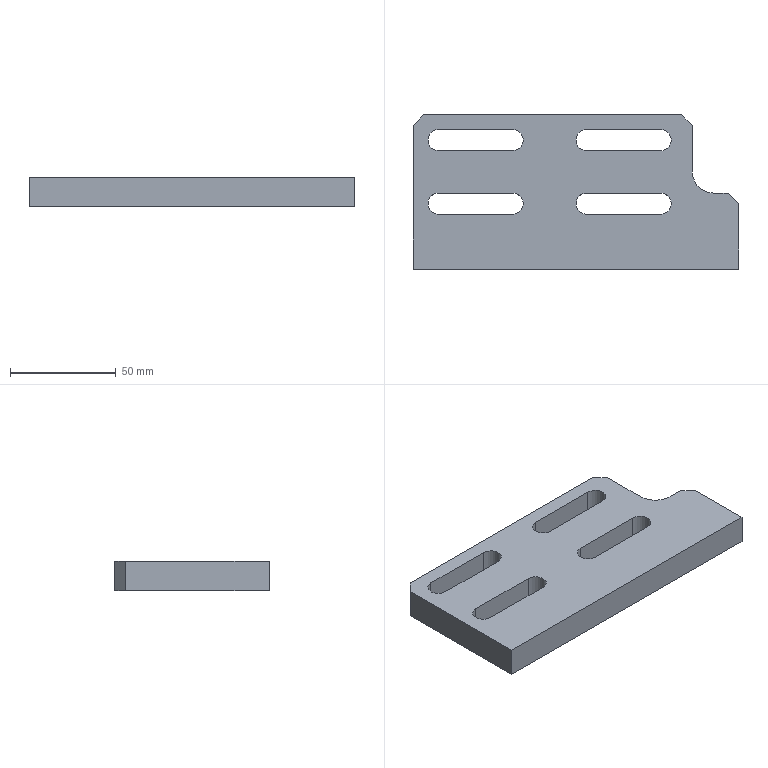Part | STEP file | [02] | 1 solid | 28 faces | box 154 x 73 x 14 mm | volume 121769 mm3 | plane 19 | cylinder 9 | commonest cylinder face diameters 10 x8 20 x1
STEP:
#1=CARTESIAN_POINT('',(15.,66.,14.));
#2=VERTEX_POINT('',#1);
#3=CARTESIAN_POINT('',(50.,66.,14.));
#4=VERTEX_POINT('',#3);
#5=CARTESIAN_POINT('',(32.5,66.,14.));
#6=DIRECTION('',(1.,0.,0.));
#7=VECTOR('',#6,1000.);
#8=LINE('',#5,#7);
#9=EDGE_CURVE('',#2,#4,#8,.T.);
#10=ORIENTED_EDGE('',*,*,#9,.T.);
#11=CARTESIAN_POINT('',(50.,56.,14.));
#12=VERTEX_POINT('',#11);
#13=CARTESIAN_POINT('',(50.,61.,14.));
#14=DIRECTION('',(0.,0.,-1.));
#15=DIRECTION('',(0.,1.,0.));
#16=AXIS2_PLACEMENT_3D('',#13,#14,#15);
#17=CIRCLE('',#16,5.);
#18=EDGE_CURVE('',#4,#12,#17,.T.);
#19=ORIENTED_EDGE('',*,*,#18,.T.);
#20=CARTESIAN_POINT('',(15.,56.,14.));
#21=VERTEX_POINT('',#20);
#22=CARTESIAN_POINT('',(32.5,56.,14.));
#23=DIRECTION('',(-1.,0.,0.));
#24=VECTOR('',#23,1000.);
#25=LINE('',#22,#24);
#26=EDGE_CURVE('',#12,#21,#25,.T.);
#27=ORIENTED_EDGE('',*,*,#26,.T.);
#28=CARTESIAN_POINT('',(15.,61.,14.));
#29=DIRECTION('',(0.,0.,-1.));
#30=DIRECTION('',(0.,1.,0.));
#31=AXIS2_PLACEMENT_3D('',#28,#29,#30);
#32=CIRCLE('',#31,5.);
#33=EDGE_CURVE('',#21,#2,#32,.T.);
#34=ORIENTED_EDGE('',*,*,#33,.T.);
#35=EDGE_LOOP('',(#10,#19,#27,#34));
#36=FACE_BOUND('',#35,.T.);
#37=CARTESIAN_POINT('',(15.,36.,14.));
#38=VERTEX_POINT('',#37);
#39=CARTESIAN_POINT('',(50.,36.,14.));
#40=VERTEX_POINT('',#39);
#41=CARTESIAN_POINT('',(32.5,36.,14.));
#42=DIRECTION('',(1.,0.,0.));
#43=VECTOR('',#42,1000.);
#44=LINE('',#41,#43);
#45=EDGE_CURVE('',#38,#40,#44,.T.);
#46=ORIENTED_EDGE('',*,*,#45,.T.);
#47=CARTESIAN_POINT('',(50.,26.,14.));
#48=VERTEX_POINT('',#47);
#49=CARTESIAN_POINT('',(50.,31.,14.));
#50=DIRECTION('',(0.,0.,-1.));
#51=DIRECTION('',(0.,1.,0.));
#52=AXIS2_PLACEMENT_3D('',#49,#50,#51);
#53=CIRCLE('',#52,5.);
#54=EDGE_CURVE('',#40,#48,#53,.T.);
#55=ORIENTED_EDGE('',*,*,#54,.T.);
#56=CARTESIAN_POINT('',(15.,26.,14.));
#57=VERTEX_POINT('',#56);
#58=CARTESIAN_POINT('',(32.5,26.,14.));
#59=DIRECTION('',(-1.,0.,0.));
#60=VECTOR('',#59,1000.);
#61=LINE('',#58,#60);
#62=EDGE_CURVE('',#48,#57,#61,.T.);
#63=ORIENTED_EDGE('',*,*,#62,.T.);
#64=CARTESIAN_POINT('',(15.,31.,14.));
#65=DIRECTION('',(0.,0.,-1.));
#66=DIRECTION('',(0.,1.,0.));
#67=AXIS2_PLACEMENT_3D('',#64,#65,#66);
#68=CIRCLE('',#67,5.);
#69=EDGE_CURVE('',#57,#38,#68,.T.);
#70=ORIENTED_EDGE('',*,*,#69,.T.);
#71=EDGE_LOOP('',(#46,#55,#63,#70));
#72=FACE_BOUND('',#71,.T.);
#73=CARTESIAN_POINT('',(85.,66.,14.));
#74=VERTEX_POINT('',#73);
#75=CARTESIAN_POINT('',(120.,66.,14.));
#76=VERTEX_POINT('',#75);
#77=CARTESIAN_POINT('',(102.5,66.,14.));
#78=DIRECTION('',(1.,0.,0.));
#79=VECTOR('',#78,1000.);
#80=LINE('',#77,#79);
#81=EDGE_CURVE('',#74,#76,#80,.T.);
#82=ORIENTED_EDGE('',*,*,#81,.T.);
#83=CARTESIAN_POINT('',(120.,56.,14.));
#84=VERTEX_POINT('',#83);
#85=CARTESIAN_POINT('',(120.,61.,14.));
#86=DIRECTION('',(0.,0.,-1.));
#87=DIRECTION('',(0.,1.,0.));
#88=AXIS2_PLACEMENT_3D('',#85,#86,#87);
#89=CIRCLE('',#88,5.);
#90=EDGE_CURVE('',#76,#84,#89,.T.);
#91=ORIENTED_EDGE('',*,*,#90,.T.);
#92=CARTESIAN_POINT('',(85.,56.,14.));
#93=VERTEX_POINT('',#92);
#94=CARTESIAN_POINT('',(102.5,56.,14.));
#95=DIRECTION('',(-1.,0.,0.));
#96=VECTOR('',#95,1000.);
#97=LINE('',#94,#96);
#98=EDGE_CURVE('',#84,#93,#97,.T.);
#99=ORIENTED_EDGE('',*,*,#98,.T.);
#100=CARTESIAN_POINT('',(85.,61.,14.));
#101=DIRECTION('',(0.,0.,-1.));
#102=DIRECTION('',(0.,1.,0.));
#103=AXIS2_PLACEMENT_3D('',#100,#101,#102);
#104=CIRCLE('',#103,5.);
#105=EDGE_CURVE('',#93,#74,#104,.T.);
#106=ORIENTED_EDGE('',*,*,#105,.T.);
#107=EDGE_LOOP('',(#82,#91,#99,#106));
#108=FACE_BOUND('',#107,.T.);
#109=CARTESIAN_POINT('',(85.,36.,14.));
#110=VERTEX_POINT('',#109);
#111=CARTESIAN_POINT('',(120.,36.,14.));
#112=VERTEX_POINT('',#111);
#113=CARTESIAN_POINT('',(102.5,36.,14.));
#114=DIRECTION('',(1.,0.,0.));
#115=VECTOR('',#114,1000.);
#116=LINE('',#113,#115);
#117=EDGE_CURVE('',#110,#112,#116,.T.);
#118=ORIENTED_EDGE('',*,*,#117,.T.);
#119=CARTESIAN_POINT('',(120.,26.,14.));
#120=VERTEX_POINT('',#119);
#121=CARTESIAN_POINT('',(120.,31.,14.));
#122=DIRECTION('',(0.,0.,-1.));
#123=DIRECTION('',(0.,1.,0.));
#124=AXIS2_PLACEMENT_3D('',#121,#122,#123);
#125=CIRCLE('',#124,5.);
#126=EDGE_CURVE('',#112,#120,#125,.T.);
#127=ORIENTED_EDGE('',*,*,#126,.T.);
#128=CARTESIAN_POINT('',(85.,26.,14.));
#129=VERTEX_POINT('',#128);
#130=CARTESIAN_POINT('',(102.5,26.,14.));
#131=DIRECTION('',(-1.,0.,0.));
#132=VECTOR('',#131,1000.);
#133=LINE('',#130,#132);
#134=EDGE_CURVE('',#120,#129,#133,.T.);
#135=ORIENTED_EDGE('',*,*,#134,.T.);
#136=CARTESIAN_POINT('',(85.,31.,14.));
#137=DIRECTION('',(0.,0.,-1.));
#138=DIRECTION('',(0.,1.,0.));
#139=AXIS2_PLACEMENT_3D('',#136,#137,#138);
#140=CIRCLE('',#139,5.);
#141=EDGE_CURVE('',#129,#110,#140,.T.);
#142=ORIENTED_EDGE('',*,*,#141,.T.);
#143=EDGE_LOOP('',(#118,#127,#135,#142));
#144=FACE_BOUND('',#143,.T.);
#145=CARTESIAN_POINT('',(135.,46.,14.));
#146=VERTEX_POINT('',#145);
#147=CARTESIAN_POINT('',(135.,68.,14.));
#148=VERTEX_POINT('',#147);
#149=CARTESIAN_POINT('',(135.,54.5,14.));
#150=DIRECTION('',(0.,1.,0.));
#151=VECTOR('',#150,1000.);
#152=LINE('',#149,#151);
#153=EDGE_CURVE('',#146,#148,#152,.T.);
#154=ORIENTED_EDGE('',*,*,#153,.T.);
#155=CARTESIAN_POINT('',(130.,73.,14.));
#156=VERTEX_POINT('',#155);
#157=CARTESIAN_POINT('',(123.25,79.75,14.));
#158=DIRECTION('',(-0.7071,0.7071,0.));
#159=VECTOR('',#158,1000.);
#160=LINE('',#157,#159);
#161=EDGE_CURVE('',#148,#156,#160,.T.);
#162=ORIENTED_EDGE('',*,*,#161,.T.);
#163=CARTESIAN_POINT('',(8.,73.,14.));
#164=VERTEX_POINT('',#163);
#165=CARTESIAN_POINT('',(80.,73.,14.));
#166=DIRECTION('',(1.,0.,0.));
#167=VECTOR('',#166,1000.);
#168=LINE('',#165,#167);
#169=EDGE_CURVE('',#164,#156,#168,.T.);
#170=ORIENTED_EDGE('',*,*,#169,.F.);
#171=CARTESIAN_POINT('',(3.,68.,14.));
#172=VERTEX_POINT('',#171);
#173=CARTESIAN_POINT('',(25.75,90.75,14.));
#174=DIRECTION('',(-0.7071,-0.7071,0.));
#175=VECTOR('',#174,1000.);
#176=LINE('',#173,#175);
#177=EDGE_CURVE('',#164,#172,#176,.T.);
#178=ORIENTED_EDGE('',*,*,#177,.T.);
#179=CARTESIAN_POINT('',(3.,0.,14.));
#180=VERTEX_POINT('',#179);
#181=CARTESIAN_POINT('',(3.,36.5,14.));
#182=DIRECTION('',(0.,1.,0.));
#183=VECTOR('',#182,1000.);
#184=LINE('',#181,#183);
#185=EDGE_CURVE('',#180,#172,#184,.T.);
#186=ORIENTED_EDGE('',*,*,#185,.F.);
#187=CARTESIAN_POINT('',(157.,0.,14.));
#188=VERTEX_POINT('',#187);
#189=CARTESIAN_POINT('',(80.,0.,14.));
#190=DIRECTION('',(-1.,0.,0.));
#191=VECTOR('',#190,1000.);
#192=LINE('',#189,#191);
#193=EDGE_CURVE('',#188,#180,#192,.T.);
#194=ORIENTED_EDGE('',*,*,#193,.F.);
#195=CARTESIAN_POINT('',(157.,31.,14.));
#196=VERTEX_POINT('',#195);
#197=CARTESIAN_POINT('',(157.,36.5,14.));
#198=DIRECTION('',(0.,-1.,0.));
#199=VECTOR('',#198,1000.);
#200=LINE('',#197,#199);
#201=EDGE_CURVE('',#196,#188,#200,.T.);
#202=ORIENTED_EDGE('',*,*,#201,.F.);
#203=CARTESIAN_POINT('',(152.,36.,14.));
#204=VERTEX_POINT('',#203);
#205=CARTESIAN_POINT('',(115.75,72.25,14.));
#206=DIRECTION('',(-0.7071,0.7071,0.));
#207=VECTOR('',#206,1000.);
#208=LINE('',#205,#207);
#209=EDGE_CURVE('',#196,#204,#208,.T.);
#210=ORIENTED_EDGE('',*,*,#209,.T.);
#211=CARTESIAN_POINT('',(145.,36.,14.));
#212=VERTEX_POINT('',#211);
#213=CARTESIAN_POINT('',(146.,36.,14.));
#214=DIRECTION('',(-1.,0.,0.));
#215=VECTOR('',#214,1000.);
#216=LINE('',#213,#215);
#217=EDGE_CURVE('',#204,#212,#216,.T.);
#218=ORIENTED_EDGE('',*,*,#217,.T.);
#219=CARTESIAN_POINT('',(145.,46.,14.));
#220=DIRECTION('',(0.,0.,-1.));
#221=DIRECTION('',(0.,-1.,0.));
#222=AXIS2_PLACEMENT_3D('',#219,#220,#221);
#223=CIRCLE('',#222,10.);
#224=EDGE_CURVE('',#212,#146,#223,.T.);
#225=ORIENTED_EDGE('',*,*,#224,.T.);
#226=EDGE_LOOP('',(#154,#162,#170,#178,#186,#194,#202,#210,#218,#225));
#227=FACE_OUTER_BOUND('',#226,.T.);
#228=CARTESIAN_POINT('',(80.,36.5,14.));
#229=DIRECTION('',(0.,0.,1.));
#230=DIRECTION('',(0.,-1.,0.));
#231=AXIS2_PLACEMENT_3D('',#228,#229,#230);
#232=PLANE('',#231);
#233=ADVANCED_FACE('',(#36,#72,#108,#144,#227),#232,.T.);
#234=CARTESIAN_POINT('',(15.,56.,0.));
#235=VERTEX_POINT('',#234);
#236=CARTESIAN_POINT('',(50.,56.,0.));
#237=VERTEX_POINT('',#236);
#238=CARTESIAN_POINT('',(32.5,56.,0.));
#239=DIRECTION('',(1.,0.,0.));
#240=VECTOR('',#239,1000.);
#241=LINE('',#238,#240);
#242=EDGE_CURVE('',#235,#237,#241,.T.);
#243=ORIENTED_EDGE('',*,*,#242,.T.);
#244=CARTESIAN_POINT('',(50.,66.,0.));
#245=VERTEX_POINT('',#244);
#246=CARTESIAN_POINT('',(50.,61.,0.));
#247=DIRECTION('',(0.,0.,1.));
#248=DIRECTION('',(0.,-1.,0.));
#249=AXIS2_PLACEMENT_3D('',#246,#247,#248);
#250=CIRCLE('',#249,5.);
#251=EDGE_CURVE('',#237,#245,#250,.T.);
#252=ORIENTED_EDGE('',*,*,#251,.T.);
#253=CARTESIAN_POINT('',(15.,66.,0.));
#254=VERTEX_POINT('',#253);
#255=CARTESIAN_POINT('',(32.5,66.,0.));
#256=DIRECTION('',(-1.,0.,0.));
#257=VECTOR('',#256,1000.);
#258=LINE('',#255,#257);
#259=EDGE_CURVE('',#245,#254,#258,.T.);
#260=ORIENTED_EDGE('',*,*,#259,.T.);
#261=CARTESIAN_POINT('',(15.,61.,0.));
#262=DIRECTION('',(0.,0.,1.));
#263=DIRECTION('',(0.,-1.,0.));
#264=AXIS2_PLACEMENT_3D('',#261,#262,#263);
#265=CIRCLE('',#264,5.);
#266=EDGE_CURVE('',#254,#235,#265,.T.);
#267=ORIENTED_EDGE('',*,*,#266,.T.);
#268=EDGE_LOOP('',(#243,#252,#260,#267));
#269=FACE_BOUND('',#268,.T.);
#270=CARTESIAN_POINT('',(15.,26.,0.));
#271=VERTEX_POINT('',#270);
#272=CARTESIAN_POINT('',(50.,26.,0.));
#273=VERTEX_POINT('',#272);
#274=CARTESIAN_POINT('',(32.5,26.,0.));
#275=DIRECTION('',(1.,0.,0.));
#276=VECTOR('',#275,1000.);
#277=LINE('',#274,#276);
#278=EDGE_CURVE('',#271,#273,#277,.T.);
#279=ORIENTED_EDGE('',*,*,#278,.T.);
#280=CARTESIAN_POINT('',(50.,36.,0.));
#281=VERTEX_POINT('',#280);
#282=CARTESIAN_POINT('',(50.,31.,0.));
#283=DIRECTION('',(0.,0.,1.));
#284=DIRECTION('',(0.,-1.,0.));
#285=AXIS2_PLACEMENT_3D('',#282,#283,#284);
#286=CIRCLE('',#285,5.);
#287=EDGE_CURVE('',#273,#281,#286,.T.);
#288=ORIENTED_EDGE('',*,*,#287,.T.);
#289=CARTESIAN_POINT('',(15.,36.,0.));
#290=VERTEX_POINT('',#289);
#291=CARTESIAN_POINT('',(32.5,36.,0.));
#292=DIRECTION('',(-1.,0.,0.));
#293=VECTOR('',#292,1000.);
#294=LINE('',#291,#293);
#295=EDGE_CURVE('',#281,#290,#294,.T.);
#296=ORIENTED_EDGE('',*,*,#295,.T.);
#297=CARTESIAN_POINT('',(15.,31.,0.));
#298=DIRECTION('',(0.,0.,1.));
#299=DIRECTION('',(0.,-1.,0.));
#300=AXIS2_PLACEMENT_3D('',#297,#298,#299);
#301=CIRCLE('',#300,5.);
#302=EDGE_CURVE('',#290,#271,#301,.T.);
#303=ORIENTED_EDGE('',*,*,#302,.T.);
#304=EDGE_LOOP('',(#279,#288,#296,#303));
#305=FACE_BOUND('',#304,.T.);
#306=CARTESIAN_POINT('',(85.,56.,0.));
#307=VERTEX_POINT('',#306);
#308=CARTESIAN_POINT('',(120.,56.,0.));
#309=VERTEX_POINT('',#308);
#310=CARTESIAN_POINT('',(102.5,56.,0.));
#311=DIRECTION('',(1.,0.,0.));
#312=VECTOR('',#311,1000.);
#313=LINE('',#310,#312);
#314=EDGE_CURVE('',#307,#309,#313,.T.);
#315=ORIENTED_EDGE('',*,*,#314,.T.);
#316=CARTESIAN_POINT('',(120.,66.,0.));
#317=VERTEX_POINT('',#316);
#318=CARTESIAN_POINT('',(120.,61.,0.));
#319=DIRECTION('',(0.,0.,1.));
#320=DIRECTION('',(0.,-1.,0.));
#321=AXIS2_PLACEMENT_3D('',#318,#319,#320);
#322=CIRCLE('',#321,5.);
#323=EDGE_CURVE('',#309,#317,#322,.T.);
#324=ORIENTED_EDGE('',*,*,#323,.T.);
#325=CARTESIAN_POINT('',(85.,66.,0.));
#326=VERTEX_POINT('',#325);
#327=CARTESIAN_POINT('',(102.5,66.,0.));
#328=DIRECTION('',(-1.,0.,0.));
#329=VECTOR('',#328,1000.);
#330=LINE('',#327,#329);
#331=EDGE_CURVE('',#317,#326,#330,.T.);
#332=ORIENTED_EDGE('',*,*,#331,.T.);
#333=CARTESIAN_POINT('',(85.,61.,0.));
#334=DIRECTION('',(0.,0.,1.));
#335=DIRECTION('',(0.,-1.,0.));
#336=AXIS2_PLACEMENT_3D('',#333,#334,#335);
#337=CIRCLE('',#336,5.);
#338=EDGE_CURVE('',#326,#307,#337,.T.);
#339=ORIENTED_EDGE('',*,*,#338,.T.);
#340=EDGE_LOOP('',(#315,#324,#332,#339));
#341=FACE_BOUND('',#340,.T.);
#342=CARTESIAN_POINT('',(85.,26.,0.));
#343=VERTEX_POINT('',#342);
#344=CARTESIAN_POINT('',(120.,26.,0.));
#345=VERTEX_POINT('',#344);
#346=CARTESIAN_POINT('',(102.5,26.,0.));
#347=DIRECTION('',(1.,0.,0.));
#348=VECTOR('',#347,1000.);
#349=LINE('',#346,#348);
#350=EDGE_CURVE('',#343,#345,#349,.T.);
#351=ORIENTED_EDGE('',*,*,#350,.T.);
#352=CARTESIAN_POINT('',(120.,36.,0.));
#353=VERTEX_POINT('',#352);
#354=CARTESIAN_POINT('',(120.,31.,0.));
#355=DIRECTION('',(0.,0.,1.));
#356=DIRECTION('',(0.,-1.,0.));
#357=AXIS2_PLACEMENT_3D('',#354,#355,#356);
#358=CIRCLE('',#357,5.);
#359=EDGE_CURVE('',#345,#353,#358,.T.);
#360=ORIENTED_EDGE('',*,*,#359,.T.);
#361=CARTESIAN_POINT('',(85.,36.,0.));
#362=VERTEX_POINT('',#361);
#363=CARTESIAN_POINT('',(102.5,36.,0.));
#364=DIRECTION('',(-1.,0.,0.));
#365=VECTOR('',#364,1000.);
#366=LINE('',#363,#365);
#367=EDGE_CURVE('',#353,#362,#366,.T.);
#368=ORIENTED_EDGE('',*,*,#367,.T.);
#369=CARTESIAN_POINT('',(85.,31.,0.));
#370=DIRECTION('',(0.,0.,1.));
#371=DIRECTION('',(0.,-1.,0.));
#372=AXIS2_PLACEMENT_3D('',#369,#370,#371);
#373=CIRCLE('',#372,5.);
#374=EDGE_CURVE('',#362,#343,#373,.T.);
#375=ORIENTED_EDGE('',*,*,#374,.T.);
#376=EDGE_LOOP('',(#351,#360,#368,#375));
#377=FACE_BOUND('',#376,.T.);
#378=CARTESIAN_POINT('',(130.,73.,0.));
#379=VERTEX_POINT('',#378);
#380=CARTESIAN_POINT('',(8.,73.,0.));
#381=VERTEX_POINT('',#380);
#382=CARTESIAN_POINT('',(80.,73.,0.));
#383=DIRECTION('',(-1.,0.,0.));
#384=VECTOR('',#383,1000.);
#385=LINE('',#382,#384);
#386=EDGE_CURVE('',#379,#381,#385,.T.);
#387=ORIENTED_EDGE('',*,*,#386,.F.);
#388=CARTESIAN_POINT('',(135.,68.,0.));
#389=VERTEX_POINT('',#388);
#390=CARTESIAN_POINT('',(123.25,79.75,0.));
#391=DIRECTION('',(0.7071,-0.7071,0.));
#392=VECTOR('',#391,1000.);
#393=LINE('',#390,#392);
#394=EDGE_CURVE('',#379,#389,#393,.T.);
#395=ORIENTED_EDGE('',*,*,#394,.T.);
#396=CARTESIAN_POINT('',(135.,46.,0.));
#397=VERTEX_POINT('',#396);
#398=CARTESIAN_POINT('',(135.,54.5,0.));
#399=DIRECTION('',(0.,-1.,0.));
#400=VECTOR('',#399,1000.);
#401=LINE('',#398,#400);
#402=EDGE_CURVE('',#389,#397,#401,.T.);
#403=ORIENTED_EDGE('',*,*,#402,.T.);
#404=CARTESIAN_POINT('',(145.,36.,0.));
#405=VERTEX_POINT('',#404);
#406=CARTESIAN_POINT('',(145.,46.,0.));
#407=DIRECTION('',(0.,0.,1.));
#408=DIRECTION('',(0.,1.,0.));
#409=AXIS2_PLACEMENT_3D('',#406,#407,#408);
#410=CIRCLE('',#409,10.);
#411=EDGE_CURVE('',#397,#405,#410,.T.);
#412=ORIENTED_EDGE('',*,*,#411,.T.);
#413=CARTESIAN_POINT('',(152.,36.,0.));
#414=VERTEX_POINT('',#413);
#415=CARTESIAN_POINT('',(146.,36.,0.));
#416=DIRECTION('',(1.,0.,0.));
#417=VECTOR('',#416,1000.);
#418=LINE('',#415,#417);
#419=EDGE_CURVE('',#405,#414,#418,.T.);
#420=ORIENTED_EDGE('',*,*,#419,.T.);
#421=CARTESIAN_POINT('',(157.,31.,0.));
#422=VERTEX_POINT('',#421);
#423=CARTESIAN_POINT('',(115.75,72.25,0.));
#424=DIRECTION('',(0.7071,-0.7071,0.));
#425=VECTOR('',#424,1000.);
#426=LINE('',#423,#425);
#427=EDGE_CURVE('',#414,#422,#426,.T.);
#428=ORIENTED_EDGE('',*,*,#427,.T.);
#429=CARTESIAN_POINT('',(157.,0.,0.));
#430=VERTEX_POINT('',#429);
#431=CARTESIAN_POINT('',(157.,36.5,0.));
#432=DIRECTION('',(0.,1.,0.));
#433=VECTOR('',#432,1000.);
#434=LINE('',#431,#433);
#435=EDGE_CURVE('',#430,#422,#434,.T.);
#436=ORIENTED_EDGE('',*,*,#435,.F.);
#437=CARTESIAN_POINT('',(3.,0.,0.));
#438=VERTEX_POINT('',#437);
#439=CARTESIAN_POINT('',(80.,0.,0.));
#440=DIRECTION('',(1.,0.,0.));
#441=VECTOR('',#440,1000.);
#442=LINE('',#439,#441);
#443=EDGE_CURVE('',#438,#430,#442,.T.);
#444=ORIENTED_EDGE('',*,*,#443,.F.);
#445=CARTESIAN_POINT('',(3.,68.,0.));
#446=VERTEX_POINT('',#445);
#447=CARTESIAN_POINT('',(3.,36.5,0.));
#448=DIRECTION('',(0.,-1.,0.));
#449=VECTOR('',#448,1000.);
#450=LINE('',#447,#449);
#451=EDGE_CURVE('',#446,#438,#450,.T.);
#452=ORIENTED_EDGE('',*,*,#451,.F.);
#453=CARTESIAN_POINT('',(25.75,90.75,0.));
#454=DIRECTION('',(0.7071,0.7071,0.));
#455=VECTOR('',#454,1000.);
#456=LINE('',#453,#455);
#457=EDGE_CURVE('',#446,#381,#456,.T.);
#458=ORIENTED_EDGE('',*,*,#457,.T.);
#459=EDGE_LOOP('',(#387,#395,#403,#412,#420,#428,#436,#444,#452,#458));
#460=FACE_OUTER_BOUND('',#459,.T.);
#461=CARTESIAN_POINT('',(80.,36.5,0.));
#462=DIRECTION('',(0.,0.,-1.));
#463=DIRECTION('',(0.,1.,0.));
#464=AXIS2_PLACEMENT_3D('',#461,#462,#463);
#465=PLANE('',#464);
#466=ADVANCED_FACE('',(#269,#305,#341,#377,#460),#465,.T.);
#467=ORIENTED_EDGE('',*,*,#435,.T.);
#468=CARTESIAN_POINT('',(157.,31.,14.));
#469=DIRECTION('',(0.,0.,1.));
#470=VECTOR('',#469,1000.);
#471=LINE('',#468,#470);
#472=EDGE_CURVE('',#422,#196,#471,.T.);
#473=ORIENTED_EDGE('',*,*,#472,.T.);
#474=ORIENTED_EDGE('',*,*,#201,.T.);
#475=CARTESIAN_POINT('',(157.,0.,0.));
#476=DIRECTION('',(0.,0.,1.));
#477=VECTOR('',#476,1000.);
#478=LINE('',#475,#477);
#479=EDGE_CURVE('',#430,#188,#478,.T.);
#480=ORIENTED_EDGE('',*,*,#479,.F.);
#481=EDGE_LOOP('',(#467,#473,#474,#480));
#482=FACE_OUTER_BOUND('',#481,.T.);
#483=CARTESIAN_POINT('',(157.,36.5,0.));
#484=DIRECTION('',(1.,0.,0.));
#485=DIRECTION('',(0.,0.,1.));
#486=AXIS2_PLACEMENT_3D('',#483,#484,#485);
#487=PLANE('',#486);
#488=ADVANCED_FACE('',(#482),#487,.T.);
#489=ORIENTED_EDGE('',*,*,#185,.T.);
#490=CARTESIAN_POINT('',(3.,68.,0.));
#491=DIRECTION('',(0.,0.,-1.));
#492=VECTOR('',#491,1000.);
#493=LINE('',#490,#492);
#494=EDGE_CURVE('',#172,#446,#493,.T.);
#495=ORIENTED_EDGE('',*,*,#494,.T.);
#496=ORIENTED_EDGE('',*,*,#451,.T.);
#497=CARTESIAN_POINT('',(3.,0.,0.));
#498=DIRECTION('',(0.,0.,1.));
#499=VECTOR('',#498,1000.);
#500=LINE('',#497,#499);
#501=EDGE_CURVE('',#438,#180,#500,.T.);
#502=ORIENTED_EDGE('',*,*,#501,.T.);
#503=EDGE_LOOP('',(#489,#495,#496,#502));
#504=FACE_OUTER_BOUND('',#503,.T.);
#505=CARTESIAN_POINT('',(3.,36.5,0.));
#506=DIRECTION('',(-1.,0.,0.));
#507=DIRECTION('',(0.,0.,-1.));
#508=AXIS2_PLACEMENT_3D('',#505,#506,#507);
#509=PLANE('',#508);
#510=ADVANCED_FACE('',(#504),#509,.T.);
#511=ORIENTED_EDGE('',*,*,#169,.T.);
#512=CARTESIAN_POINT('',(130.,73.,0.));
#513=DIRECTION('',(0.,0.,-1.));
#514=VECTOR('',#513,1000.);
#515=LINE('',#512,#514);
#516=EDGE_CURVE('',#156,#379,#515,.T.);
#517=ORIENTED_EDGE('',*,*,#516,.T.);
#518=ORIENTED_EDGE('',*,*,#386,.T.);
#519=CARTESIAN_POINT('',(8.,73.,0.));
#520=DIRECTION('',(0.,0.,1.));
#521=VECTOR('',#520,1000.);
#522=LINE('',#519,#521);
#523=EDGE_CURVE('',#381,#164,#522,.T.);
#524=ORIENTED_EDGE('',*,*,#523,.T.);
#525=EDGE_LOOP('',(#511,#517,#518,#524));
#526=FACE_OUTER_BOUND('',#525,.T.);
#527=CARTESIAN_POINT('',(80.,73.,0.));
#528=DIRECTION('',(0.,1.,0.));
#529=DIRECTION('',(0.,0.,1.));
#530=AXIS2_PLACEMENT_3D('',#527,#528,#529);
#531=PLANE('',#530);
#532=ADVANCED_FACE('',(#526),#531,.T.);
#533=ORIENTED_EDGE('',*,*,#443,.T.);
#534=ORIENTED_EDGE('',*,*,#479,.T.);
#535=ORIENTED_EDGE('',*,*,#193,.T.);
#536=ORIENTED_EDGE('',*,*,#501,.F.);
#537=EDGE_LOOP('',(#533,#534,#535,#536));
#538=FACE_OUTER_BOUND('',#537,.T.);
#539=CARTESIAN_POINT('',(80.,0.,0.));
#540=DIRECTION('',(0.,-1.,0.));
#541=DIRECTION('',(0.,0.,-1.));
#542=AXIS2_PLACEMENT_3D('',#539,#540,#541);
#543=PLANE('',#542);
#544=ADVANCED_FACE('',(#538),#543,.T.);
#545=ORIENTED_EDGE('',*,*,#457,.F.);
#546=ORIENTED_EDGE('',*,*,#494,.F.);
#547=ORIENTED_EDGE('',*,*,#177,.F.);
#548=ORIENTED_EDGE('',*,*,#523,.F.);
#549=EDGE_LOOP('',(#545,#546,#547,#548));
#550=FACE_OUTER_BOUND('',#549,.T.);
#551=CARTESIAN_POINT('',(8.,73.,0.));
#552=DIRECTION('',(0.7071,-0.7071,0.));
#553=DIRECTION('',(0.,0.,1.));
#554=AXIS2_PLACEMENT_3D('',#551,#552,#553);
#555=PLANE('',#554);
#556=ADVANCED_FACE('',(#550),#555,.F.);
#557=CARTESIAN_POINT('',(50.,56.,0.));
#558=DIRECTION('',(0.,0.,1.));
#559=VECTOR('',#558,1000.);
#560=LINE('',#557,#559);
#561=EDGE_CURVE('',#237,#12,#560,.T.);
#562=ORIENTED_EDGE('',*,*,#561,.F.);
#563=ORIENTED_EDGE('',*,*,#242,.F.);
#564=CARTESIAN_POINT('',(15.,56.,0.));
#565=DIRECTION('',(0.,0.,1.));
#566=VECTOR('',#565,1000.);
#567=LINE('',#564,#566);
#568=EDGE_CURVE('',#235,#21,#567,.T.);
#569=ORIENTED_EDGE('',*,*,#568,.T.);
#570=ORIENTED_EDGE('',*,*,#26,.F.);
#571=EDGE_LOOP('',(#562,#563,#569,#570));
#572=FACE_OUTER_BOUND('',#571,.T.);
#573=CARTESIAN_POINT('',(32.5,56.,0.));
#574=DIRECTION('',(0.,-1.,0.));
#575=DIRECTION('',(0.,0.,-1.));
#576=AXIS2_PLACEMENT_3D('',#573,#574,#575);
#577=PLANE('',#576);
#578=ADVANCED_FACE('',(#572),#577,.F.);
#579=CARTESIAN_POINT('',(15.,66.,0.));
#580=DIRECTION('',(0.,0.,1.));
#581=VECTOR('',#580,1000.);
#582=LINE('',#579,#581);
#583=EDGE_CURVE('',#254,#2,#582,.T.);
#584=ORIENTED_EDGE('',*,*,#583,.F.);
#585=ORIENTED_EDGE('',*,*,#259,.F.);
#586=CARTESIAN_POINT('',(50.,66.,0.));
#587=DIRECTION('',(0.,0.,1.));
#588=VECTOR('',#587,1000.);
#589=LINE('',#586,#588);
#590=EDGE_CURVE('',#245,#4,#589,.T.);
#591=ORIENTED_EDGE('',*,*,#590,.T.);
#592=ORIENTED_EDGE('',*,*,#9,.F.);
#593=EDGE_LOOP('',(#584,#585,#591,#592));
#594=FACE_OUTER_BOUND('',#593,.T.);
#595=CARTESIAN_POINT('',(32.5,66.,0.));
#596=DIRECTION('',(0.,1.,0.));
#597=DIRECTION('',(0.,0.,1.));
#598=AXIS2_PLACEMENT_3D('',#595,#596,#597);
#599=PLANE('',#598);
#600=ADVANCED_FACE('',(#594),#599,.F.);
#601=ORIENTED_EDGE('',*,*,#251,.F.);
#602=ORIENTED_EDGE('',*,*,#561,.T.);
#603=ORIENTED_EDGE('',*,*,#18,.F.);
#604=ORIENTED_EDGE('',*,*,#590,.F.);
#605=EDGE_LOOP('',(#601,#602,#603,#604));
#606=FACE_OUTER_BOUND('',#605,.T.);
#607=CARTESIAN_POINT('',(50.,61.,0.));
#608=DIRECTION('',(0.,0.,1.));
#609=DIRECTION('',(0.,-1.,0.));
#610=AXIS2_PLACEMENT_3D('',#607,#608,#609);
#611=CYLINDRICAL_SURFACE('',#610,5.);
#612=ADVANCED_FACE('',(#606),#611,.F.);
#613=ORIENTED_EDGE('',*,*,#266,.F.);
#614=ORIENTED_EDGE('',*,*,#583,.T.);
#615=ORIENTED_EDGE('',*,*,#33,.F.);
#616=ORIENTED_EDGE('',*,*,#568,.F.);
#617=EDGE_LOOP('',(#613,#614,#615,#616));
#618=FACE_OUTER_BOUND('',#617,.T.);
#619=CARTESIAN_POINT('',(15.,61.,0.));
#620=DIRECTION('',(0.,0.,1.));
#621=DIRECTION('',(0.,-1.,0.));
#622=AXIS2_PLACEMENT_3D('',#619,#620,#621);
#623=CYLINDRICAL_SURFACE('',#622,5.);
#624=ADVANCED_FACE('',(#618),#623,.F.);
#625=CARTESIAN_POINT('',(50.,26.,0.));
#626=DIRECTION('',(0.,0.,1.));
#627=VECTOR('',#626,1000.);
#628=LINE('',#625,#627);
#629=EDGE_CURVE('',#273,#48,#628,.T.);
#630=ORIENTED_EDGE('',*,*,#629,.F.);
#631=ORIENTED_EDGE('',*,*,#278,.F.);
#632=CARTESIAN_POINT('',(15.,26.,0.));
#633=DIRECTION('',(0.,0.,1.));
#634=VECTOR('',#633,1000.);
#635=LINE('',#632,#634);
#636=EDGE_CURVE('',#271,#57,#635,.T.);
#637=ORIENTED_EDGE('',*,*,#636,.T.);
#638=ORIENTED_EDGE('',*,*,#62,.F.);
#639=EDGE_LOOP('',(#630,#631,#637,#638));
#640=FACE_OUTER_BOUND('',#639,.T.);
#641=CARTESIAN_POINT('',(32.5,26.,0.));
#642=DIRECTION('',(0.,-1.,0.));
#643=DIRECTION('',(0.,0.,-1.));
#644=AXIS2_PLACEMENT_3D('',#641,#642,#643);
#645=PLANE('',#644);
#646=ADVANCED_FACE('',(#640),#645,.F.);
#647=CARTESIAN_POINT('',(15.,36.,0.));
#648=DIRECTION('',(0.,0.,1.));
#649=VECTOR('',#648,1000.);
#650=LINE('',#647,#649);
#651=EDGE_CURVE('',#290,#38,#650,.T.);
#652=ORIENTED_EDGE('',*,*,#651,.F.);
#653=ORIENTED_EDGE('',*,*,#295,.F.);
#654=CARTESIAN_POINT('',(50.,36.,0.));
#655=DIRECTION('',(0.,0.,1.));
#656=VECTOR('',#655,1000.);
#657=LINE('',#654,#656);
#658=EDGE_CURVE('',#281,#40,#657,.T.);
#659=ORIENTED_EDGE('',*,*,#658,.T.);
#660=ORIENTED_EDGE('',*,*,#45,.F.);
#661=EDGE_LOOP('',(#652,#653,#659,#660));
#662=FACE_OUTER_BOUND('',#661,.T.);
#663=CARTESIAN_POINT('',(32.5,36.,0.));
#664=DIRECTION('',(0.,1.,0.));
#665=DIRECTION('',(0.,0.,1.));
#666=AXIS2_PLACEMENT_3D('',#663,#664,#665);
#667=PLANE('',#666);
#668=ADVANCED_FACE('',(#662),#667,.F.);
#669=ORIENTED_EDGE('',*,*,#287,.F.);
#670=ORIENTED_EDGE('',*,*,#629,.T.);
#671=ORIENTED_EDGE('',*,*,#54,.F.);
#672=ORIENTED_EDGE('',*,*,#658,.F.);
#673=EDGE_LOOP('',(#669,#670,#671,#672));
#674=FACE_OUTER_BOUND('',#673,.T.);
#675=CARTESIAN_POINT('',(50.,31.,0.));
#676=DIRECTION('',(0.,0.,1.));
#677=DIRECTION('',(0.,-1.,0.));
#678=AXIS2_PLACEMENT_3D('',#675,#676,#677);
#679=CYLINDRICAL_SURFACE('',#678,5.);
#680=ADVANCED_FACE('',(#674),#679,.F.);
#681=ORIENTED_EDGE('',*,*,#302,.F.);
#682=ORIENTED_EDGE('',*,*,#651,.T.);
#683=ORIENTED_EDGE('',*,*,#69,.F.);
#684=ORIENTED_EDGE('',*,*,#636,.F.);
#685=EDGE_LOOP('',(#681,#682,#683,#684));
#686=FACE_OUTER_BOUND('',#685,.T.);
#687=CARTESIAN_POINT('',(15.,31.,0.));
#688=DIRECTION('',(0.,0.,1.));
#689=DIRECTION('',(0.,-1.,0.));
#690=AXIS2_PLACEMENT_3D('',#687,#688,#689);
#691=CYLINDRICAL_SURFACE('',#690,5.);
#692=ADVANCED_FACE('',(#686),#691,.F.);
#693=CARTESIAN_POINT('',(120.,56.,0.));
#694=DIRECTION('',(0.,0.,1.));
#695=VECTOR('',#694,1000.);
#696=LINE('',#693,#695);
#697=EDGE_CURVE('',#309,#84,#696,.T.);
#698=ORIENTED_EDGE('',*,*,#697,.F.);
#699=ORIENTED_EDGE('',*,*,#314,.F.);
#700=CARTESIAN_POINT('',(85.,56.,0.));
#701=DIRECTION('',(0.,0.,1.));
#702=VECTOR('',#701,1000.);
#703=LINE('',#700,#702);
#704=EDGE_CURVE('',#307,#93,#703,.T.);
#705=ORIENTED_EDGE('',*,*,#704,.T.);
#706=ORIENTED_EDGE('',*,*,#98,.F.);
#707=EDGE_LOOP('',(#698,#699,#705,#706));
#708=FACE_OUTER_BOUND('',#707,.T.);
#709=CARTESIAN_POINT('',(102.5,56.,0.));
#710=DIRECTION('',(0.,-1.,0.));
#711=DIRECTION('',(0.,0.,-1.));
#712=AXIS2_PLACEMENT_3D('',#709,#710,#711);
#713=PLANE('',#712);
#714=ADVANCED_FACE('',(#708),#713,.F.);
#715=CARTESIAN_POINT('',(85.,66.,0.));
#716=DIRECTION('',(0.,0.,1.));
#717=VECTOR('',#716,1000.);
#718=LINE('',#715,#717);
#719=EDGE_CURVE('',#326,#74,#718,.T.);
#720=ORIENTED_EDGE('',*,*,#719,.F.);
#721=ORIENTED_EDGE('',*,*,#331,.F.);
#722=CARTESIAN_POINT('',(120.,66.,0.));
#723=DIRECTION('',(0.,0.,1.));
#724=VECTOR('',#723,1000.);
#725=LINE('',#722,#724);
#726=EDGE_CURVE('',#317,#76,#725,.T.);
#727=ORIENTED_EDGE('',*,*,#726,.T.);
#728=ORIENTED_EDGE('',*,*,#81,.F.);
#729=EDGE_LOOP('',(#720,#721,#727,#728));
#730=FACE_OUTER_BOUND('',#729,.T.);
#731=CARTESIAN_POINT('',(102.5,66.,0.));
#732=DIRECTION('',(0.,1.,0.));
#733=DIRECTION('',(0.,0.,1.));
#734=AXIS2_PLACEMENT_3D('',#731,#732,#733);
#735=PLANE('',#734);
#736=ADVANCED_FACE('',(#730),#735,.F.);
#737=ORIENTED_EDGE('',*,*,#323,.F.);
#738=ORIENTED_EDGE('',*,*,#697,.T.);
#739=ORIENTED_EDGE('',*,*,#90,.F.);
#740=ORIENTED_EDGE('',*,*,#726,.F.);
#741=EDGE_LOOP('',(#737,#738,#739,#740));
#742=FACE_OUTER_BOUND('',#741,.T.);
#743=CARTESIAN_POINT('',(120.,61.,0.));
#744=DIRECTION('',(0.,0.,1.));
#745=DIRECTION('',(0.,-1.,0.));
#746=AXIS2_PLACEMENT_3D('',#743,#744,#745);
#747=CYLINDRICAL_SURFACE('',#746,5.);
#748=ADVANCED_FACE('',(#742),#747,.F.);
#749=ORIENTED_EDGE('',*,*,#338,.F.);
#750=ORIENTED_EDGE('',*,*,#719,.T.);
#751=ORIENTED_EDGE('',*,*,#105,.F.);
#752=ORIENTED_EDGE('',*,*,#704,.F.);
#753=EDGE_LOOP('',(#749,#750,#751,#752));
#754=FACE_OUTER_BOUND('',#753,.T.);
#755=CARTESIAN_POINT('',(85.,61.,0.));
#756=DIRECTION('',(0.,0.,1.));
#757=DIRECTION('',(0.,-1.,0.));
#758=AXIS2_PLACEMENT_3D('',#755,#756,#757);
#759=CYLINDRICAL_SURFACE('',#758,5.);
#760=ADVANCED_FACE('',(#754),#759,.F.);
#761=CARTESIAN_POINT('',(120.,26.,0.));
#762=DIRECTION('',(0.,0.,1.));
#763=VECTOR('',#762,1000.);
#764=LINE('',#761,#763);
#765=EDGE_CURVE('',#345,#120,#764,.T.);
#766=ORIENTED_EDGE('',*,*,#765,.F.);
#767=ORIENTED_EDGE('',*,*,#350,.F.);
#768=CARTESIAN_POINT('',(85.,26.,0.));
#769=DIRECTION('',(0.,0.,1.));
#770=VECTOR('',#769,1000.);
#771=LINE('',#768,#770);
#772=EDGE_CURVE('',#343,#129,#771,.T.);
#773=ORIENTED_EDGE('',*,*,#772,.T.);
#774=ORIENTED_EDGE('',*,*,#134,.F.);
#775=EDGE_LOOP('',(#766,#767,#773,#774));
#776=FACE_OUTER_BOUND('',#775,.T.);
#777=CARTESIAN_POINT('',(102.5,26.,0.));
#778=DIRECTION('',(0.,-1.,0.));
#779=DIRECTION('',(0.,0.,-1.));
#780=AXIS2_PLACEMENT_3D('',#777,#778,#779);
#781=PLANE('',#780);
#782=ADVANCED_FACE('',(#776),#781,.F.);
#783=CARTESIAN_POINT('',(85.,36.,0.));
#784=DIRECTION('',(0.,0.,1.));
#785=VECTOR('',#784,1000.);
#786=LINE('',#783,#785);
#787=EDGE_CURVE('',#362,#110,#786,.T.);
#788=ORIENTED_EDGE('',*,*,#787,.F.);
#789=ORIENTED_EDGE('',*,*,#367,.F.);
#790=CARTESIAN_POINT('',(120.,36.,0.));
#791=DIRECTION('',(0.,0.,1.));
#792=VECTOR('',#791,1000.);
#793=LINE('',#790,#792);
#794=EDGE_CURVE('',#353,#112,#793,.T.);
#795=ORIENTED_EDGE('',*,*,#794,.T.);
#796=ORIENTED_EDGE('',*,*,#117,.F.);
#797=EDGE_LOOP('',(#788,#789,#795,#796));
#798=FACE_OUTER_BOUND('',#797,.T.);
#799=CARTESIAN_POINT('',(102.5,36.,0.));
#800=DIRECTION('',(0.,1.,0.));
#801=DIRECTION('',(0.,0.,1.));
#802=AXIS2_PLACEMENT_3D('',#799,#800,#801);
#803=PLANE('',#802);
#804=ADVANCED_FACE('',(#798),#803,.F.);
#805=ORIENTED_EDGE('',*,*,#359,.F.);
#806=ORIENTED_EDGE('',*,*,#765,.T.);
#807=ORIENTED_EDGE('',*,*,#126,.F.);
#808=ORIENTED_EDGE('',*,*,#794,.F.);
#809=EDGE_LOOP('',(#805,#806,#807,#808));
#810=FACE_OUTER_BOUND('',#809,.T.);
#811=CARTESIAN_POINT('',(120.,31.,0.));
#812=DIRECTION('',(0.,0.,1.));
#813=DIRECTION('',(0.,-1.,0.));
#814=AXIS2_PLACEMENT_3D('',#811,#812,#813);
#815=CYLINDRICAL_SURFACE('',#814,5.);
#816=ADVANCED_FACE('',(#810),#815,.F.);
#817=ORIENTED_EDGE('',*,*,#374,.F.);
#818=ORIENTED_EDGE('',*,*,#787,.T.);
#819=ORIENTED_EDGE('',*,*,#141,.F.);
#820=ORIENTED_EDGE('',*,*,#772,.F.);
#821=EDGE_LOOP('',(#817,#818,#819,#820));
#822=FACE_OUTER_BOUND('',#821,.T.);
#823=CARTESIAN_POINT('',(85.,31.,0.));
#824=DIRECTION('',(0.,0.,1.));
#825=DIRECTION('',(0.,-1.,0.));
#826=AXIS2_PLACEMENT_3D('',#823,#824,#825);
#827=CYLINDRICAL_SURFACE('',#826,5.);
#828=ADVANCED_FACE('',(#822),#827,.F.);
#829=ORIENTED_EDGE('',*,*,#217,.F.);
#830=CARTESIAN_POINT('',(152.,36.,0.));
#831=DIRECTION('',(0.,0.,-1.));
#832=VECTOR('',#831,1000.);
#833=LINE('',#830,#832);
#834=EDGE_CURVE('',#204,#414,#833,.T.);
#835=ORIENTED_EDGE('',*,*,#834,.T.);
#836=ORIENTED_EDGE('',*,*,#419,.F.);
#837=CARTESIAN_POINT('',(145.,36.,14.));
#838=DIRECTION('',(0.,0.,1.));
#839=VECTOR('',#838,1000.);
#840=LINE('',#837,#839);
#841=EDGE_CURVE('',#405,#212,#840,.T.);
#842=ORIENTED_EDGE('',*,*,#841,.T.);
#843=EDGE_LOOP('',(#829,#835,#836,#842));
#844=FACE_OUTER_BOUND('',#843,.T.);
#845=CARTESIAN_POINT('',(146.,36.,0.));
#846=DIRECTION('',(0.,-1.,0.));
#847=DIRECTION('',(0.,0.,1.));
#848=AXIS2_PLACEMENT_3D('',#845,#846,#847);
#849=PLANE('',#848);
#850=ADVANCED_FACE('',(#844),#849,.F.);
#851=ORIENTED_EDGE('',*,*,#402,.F.);
#852=CARTESIAN_POINT('',(135.,68.,14.));
#853=DIRECTION('',(0.,0.,1.));
#854=VECTOR('',#853,1000.);
#855=LINE('',#852,#854);
#856=EDGE_CURVE('',#389,#148,#855,.T.);
#857=ORIENTED_EDGE('',*,*,#856,.T.);
#858=ORIENTED_EDGE('',*,*,#153,.F.);
#859=CARTESIAN_POINT('',(135.,46.,0.));
#860=DIRECTION('',(0.,0.,-1.));
#861=VECTOR('',#860,1000.);
#862=LINE('',#859,#861);
#863=EDGE_CURVE('',#146,#397,#862,.T.);
#864=ORIENTED_EDGE('',*,*,#863,.T.);
#865=EDGE_LOOP('',(#851,#857,#858,#864));
#866=FACE_OUTER_BOUND('',#865,.T.);
#867=CARTESIAN_POINT('',(135.,54.5,0.));
#868=DIRECTION('',(-1.,0.,0.));
#869=DIRECTION('',(0.,0.,1.));
#870=AXIS2_PLACEMENT_3D('',#867,#868,#869);
#871=PLANE('',#870);
#872=ADVANCED_FACE('',(#866),#871,.F.);
#873=ORIENTED_EDGE('',*,*,#411,.F.);
#874=ORIENTED_EDGE('',*,*,#863,.F.);
#875=ORIENTED_EDGE('',*,*,#224,.F.);
#876=ORIENTED_EDGE('',*,*,#841,.F.);
#877=EDGE_LOOP('',(#873,#874,#875,#876));
#878=FACE_OUTER_BOUND('',#877,.T.);
#879=CARTESIAN_POINT('',(145.,46.,0.));
#880=DIRECTION('',(0.,0.,-1.));
#881=DIRECTION('',(0.,1.,0.));
#882=AXIS2_PLACEMENT_3D('',#879,#880,#881);
#883=CYLINDRICAL_SURFACE('',#882,10.);
#884=ADVANCED_FACE('',(#878),#883,.F.);
#885=ORIENTED_EDGE('',*,*,#427,.F.);
#886=ORIENTED_EDGE('',*,*,#834,.F.);
#887=ORIENTED_EDGE('',*,*,#209,.F.);
#888=ORIENTED_EDGE('',*,*,#472,.F.);
#889=EDGE_LOOP('',(#885,#886,#887,#888));
#890=FACE_OUTER_BOUND('',#889,.T.);
#891=CARTESIAN_POINT('',(157.,31.,0.));
#892=DIRECTION('',(0.7071,0.7071,0.));
#893=DIRECTION('',(0.,0.,-1.));
#894=AXIS2_PLACEMENT_3D('',#891,#892,#893);
#895=PLANE('',#894);
#896=ADVANCED_FACE('',(#890),#895,.T.);
#897=ORIENTED_EDGE('',*,*,#394,.F.);
#898=ORIENTED_EDGE('',*,*,#516,.F.);
#899=ORIENTED_EDGE('',*,*,#161,.F.);
#900=ORIENTED_EDGE('',*,*,#856,.F.);
#901=EDGE_LOOP('',(#897,#898,#899,#900));
#902=FACE_OUTER_BOUND('',#901,.T.);
#903=CARTESIAN_POINT('',(135.,68.,0.));
#904=DIRECTION('',(0.7071,0.7071,0.));
#905=DIRECTION('',(0.,0.,-1.));
#906=AXIS2_PLACEMENT_3D('',#903,#904,#905);
#907=PLANE('',#906);
#908=ADVANCED_FACE('',(#902),#907,.T.);
#909=CLOSED_SHELL('',(#233,#466,#488,#510,#532,#544,#556,#578,#600,#612,#624,#646,#668,#680,#692,#714,#736,#748,#760,#782,#804,#816,#828,#850,#872,#884,#896,#908));
#910=MANIFOLD_SOLID_BREP('',#909);
#911=CARTESIAN_POINT('',(0.,0.,0.));
#912=DIRECTION('',(0.,0.,1.));
#913=DIRECTION('',(1.,0.,0.));
#914=AXIS2_PLACEMENT_3D('',#911,#912,#913);
#915=(LENGTH_UNIT()NAMED_UNIT(*)SI_UNIT(.MILLI.,.METRE.));
#916=UNCERTAINTY_MEASURE_WITH_UNIT(LENGTH_MEASURE(0.00001),#915,'','');
#917=(NAMED_UNIT(*)PLANE_ANGLE_UNIT()SI_UNIT($,.RADIAN.));
#918=(NAMED_UNIT(*)SI_UNIT($,.STERADIAN.)SOLID_ANGLE_UNIT());
#919=(GEOMETRIC_REPRESENTATION_CONTEXT(3)GLOBAL_UNCERTAINTY_ASSIGNED_CONTEXT((#916))GLOBAL_UNIT_ASSIGNED_CONTEXT((#915,#917,#918))REPRESENTATION_CONTEXT('',''));
#920=ADVANCED_BREP_SHAPE_REPRESENTATION('',(#910,#914),#919);